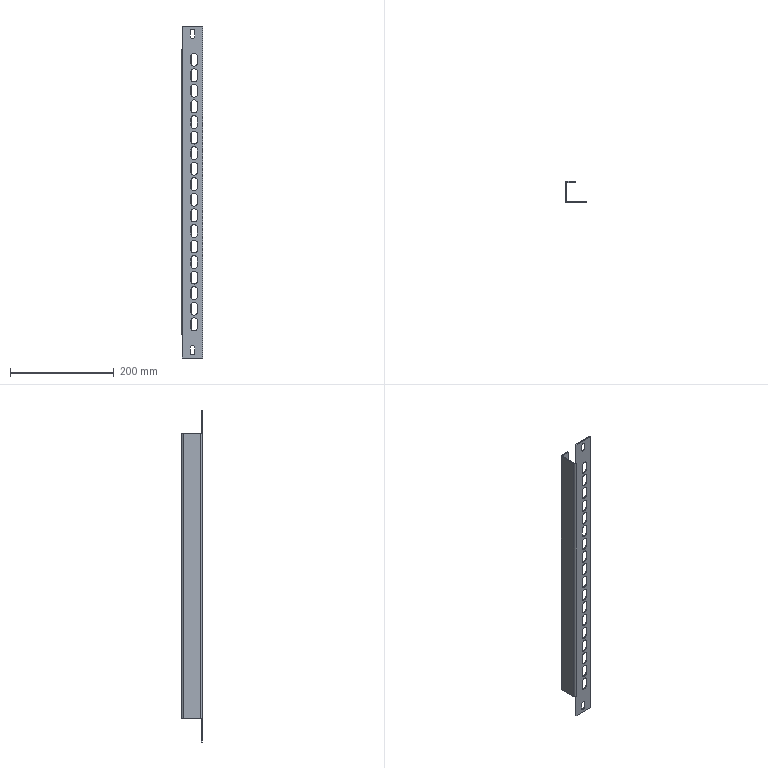Part | STEP file | 1 solid | 124 faces | box 42 x 40 x 640 mm | volume 101667 mm3 | cylinder 62 | plane 62 | commonest cylinder face diameters 13 x54 9 x4 3 x2 7 x2